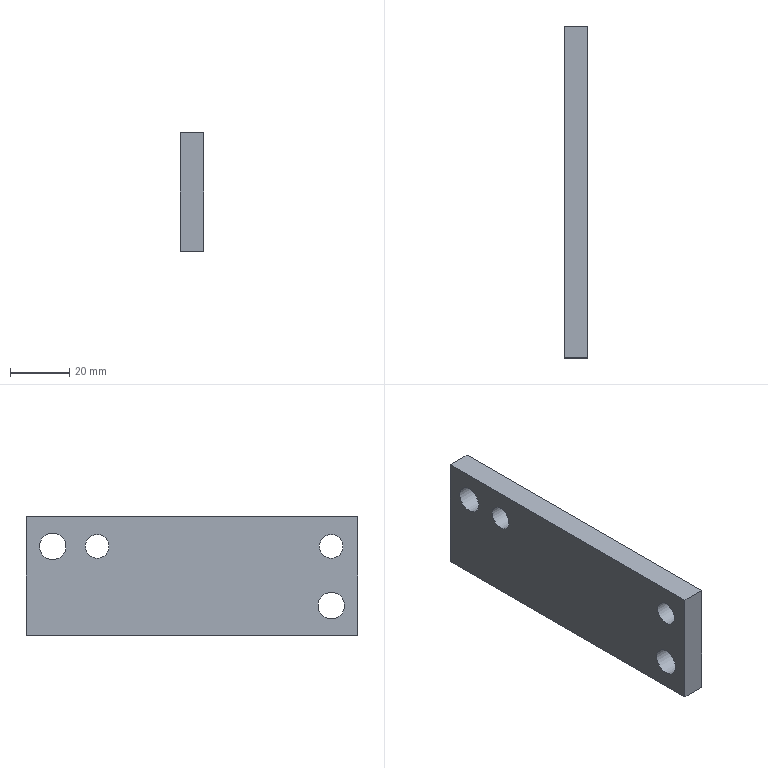Part | STEP file | solid 86 | 1 solid | 10 faces | box 8 x 112 x 40 mm | volume 34018 mm3 | plane 6 | cylinder 4 | commonest cylinder face diameters 8 x2 9 x2